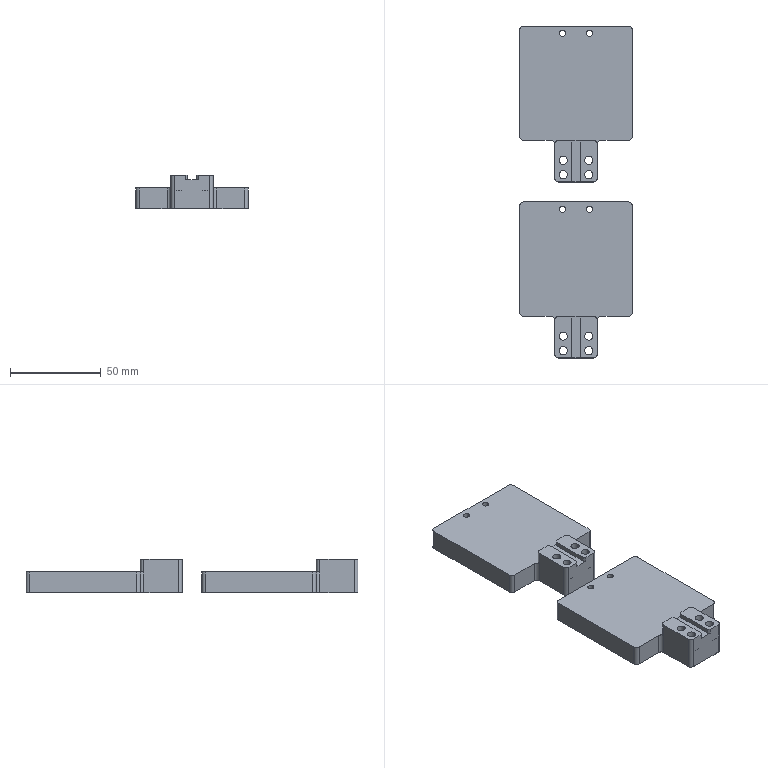NC program | NX | posted with a generic post | part box 62 x 183 x 18.5 mm
Lines 1 to 2420 of 4383, first 2274 of 2406 lines:
N10 G17 G21 G94 G90
(FLOOR_WALL , TOOL : D80)
N12 T19 M6
N14 G54
N16 G17 G0 G90 X229. Y31. S6500 M3
N18 G43 Z30. H19
N20 Z3.
N22 G94 G1 Z0. F1500.
N24 X226.
N26 X-43.
N28 X-46.
N30 Z3.
N32 G0 Z30.
N34 M5
(CAVITY_MILL , TOOL : D10)
N36 T15 M6
N38 G54
N40 G17 G0 G90 X84.33 Y-9.997 S9500 M3
N42 G43 Z30. H15
N44 Z1.026
N46 G94 G1 Z-0.974 F1000.
N48 X80.866 Y-3.997
N50 G3 X80. Y-3.497 R1.
N52 G1 X67.219 F3500.
N54 G2 X61. Y-6.3 R8.3
N56 G1 X2.
N58 G2 X-6.3 Y2. R8.3
N60 G1 Y60.
N62 G2 X2. Y68.3 R8.3
N64 G1 X61.
N66 G2 X67.219 Y65.497 R8.3
N68 G1 X90.7
N70 Y59.497
N72 Y45.599
N74 G3 X84. Y49. R8.3
N76 G1 X69.3
N78 Y59.497
N80 X90.7
N82 X86.2 Y54.997
N84 Y53.31
N86 G3 X84. Y53.5 R12.8
N88 G1 X73.8
N90 Y54.997
N92 X86.2
N94 X90.7 Y59.497
N96 Y65.497
N98 X92.781
N100 G2 X99. Y68.3 R8.3
N102 G1 X158.
N104 G2 X164.219 Y65.497 R8.3
N106 G1 X186.
N108 G2 X186.497 Y65. R0.497
N110 G1 Y49.
N112 X180.497
N114 X166.3
N116 Y59.497
N118 X180.497
N120 Y49.
N122 X175.997 Y53.5
N124 X170.8
N126 Y54.997
N128 X175.997
N130 Y53.5
N132 X180.497 Y49.
N134 X186.497
N136 Y46.919
N138 G2 X189.3 Y40.7 R8.3
N140 G1 Y21.3
N142 G2 X186.497 Y15.081 R8.3
N144 G1 Y-3.
N146 G2 X186. Y-3.497 R0.497
N148 G1 X166.3
N150 Y2.503
N152 Y13.
N154 X180.497
N156 Y2.503
N158 X166.3
N160 X170.8 Y7.003
N162 Y8.5
N164 X175.997
N166 Y7.003
N168 X170.8
N170 X166.3 Y2.503
N172 Y-3.497
N174 X164.219
N176 G2 X158. Y-6.3 R8.3
N178 G1 X99.
N180 G2 X92.781 Y-3.497 R8.3
N182 G1 X80.
N184 Y2.503
N186 X69.3
N188 Y13.
N190 X84.
N192 G3 X90.7 Y16.401 R8.3
N194 G1 X89.731 Y17.109
N196 G2 X84. Y14.2 R7.1
N198 G1 X68.1
N200 Y2.
N202 G2 X61. Y-5.1 R7.1
N204 G1 X2.
N206 G2 X-5.1 Y2. R7.1
N208 G1 Y60.
N210 G2 X2. Y67.1 R7.1
N212 G1 X61.
N214 G2 X68.1 Y60. R7.1
N216 G1 Y47.8
N218 X84.
N220 G2 X91.1 Y40.7 R7.1
N222 G1 Y21.3
N224 G2 X89.731 Y17.109 R7.1
N226 G1 X90.7 Y16.401
N228 Y2.503
N230 X91.9
N232 Y60.
N234 G2 X99. Y67.1 R7.1
N236 G1 X158.
N238 G2 X165.1 Y60. R7.1
N240 G1 Y47.8
N242 X181.
N244 G2 X188.1 Y40.7 R7.1
N246 G1 Y21.3
N248 G2 X181. Y14.2 R7.1
N250 G1 X165.1
N252 Y2.
N254 G2 X158. Y-5.1 R7.1
N256 G1 X99.
N258 G2 X91.9 Y2. R7.1
N260 G1 Y2.503
N262 X90.7
N264 X80.
N266 Y7.003
N268 X73.8
N270 Y8.5
N272 X84.
N274 G3 X86.2 Y8.69 R12.8
N276 G1 Y7.003
N278 X80.
N280 G3 X79.134 Y6.503 R1.
N282 G1 Z1.026
N284 G0 Z30.
N286 X84.33 Y-9.997
N288 Z0.053
N290 G1 Z-1.947 F1000.
N292 X80.866 Y-3.997
N294 G3 X80. Y-3.497 R1.
N296 G1 X67.219 F3500.
N298 G2 X61. Y-6.3 R8.3
N300 G1 X2.
N302 G2 X-6.3 Y2. R8.3
N304 G1 Y60.
N306 G2 X2. Y68.3 R8.3
N308 G1 X61.
N310 G2 X67.219 Y65.497 R8.3
N312 G1 X90.7
N314 Y59.497
N316 Y45.599
N318 G3 X84. Y49. R8.3
N320 G1 X69.3
N322 Y59.497
N324 X90.7
N326 X86.2 Y54.997
N328 Y53.31
N330 G3 X84. Y53.5 R12.8
N332 G1 X73.8
N334 Y54.997
N336 X86.2
N338 X90.7 Y59.497
N340 Y65.497
N342 X92.781
N344 G2 X99. Y68.3 R8.3
N346 G1 X158.
N348 G2 X164.219 Y65.497 R8.3
N350 G1 X186.
N352 G2 X186.497 Y65. R0.497
N354 G1 Y49.
N356 X180.497
N358 X166.3
N360 Y59.497
N362 X180.497
N364 Y49.
N366 X175.997 Y53.5
N368 X170.8
N370 Y54.997
N372 X175.997
N374 Y53.5
N376 X180.497 Y49.
N378 X186.497
N380 Y46.919
N382 G2 X189.3 Y40.7 R8.3
N384 G1 Y21.3
N386 G2 X186.497 Y15.081 R8.3
N388 G1 Y-3.
N390 G2 X186. Y-3.497 R0.497
N392 G1 X166.3
N394 Y2.503
N396 Y13.
N398 X180.497
N400 Y2.503
N402 X166.3
N404 X170.8 Y7.003
N406 Y8.5
N408 X175.997
N410 Y7.003
N412 X170.8
N414 X166.3 Y2.503
N416 Y-3.497
N418 X164.219
N420 G2 X158. Y-6.3 R8.3
N422 G1 X99.
N424 G2 X92.781 Y-3.497 R8.3
N426 G1 X80.
N428 Y2.503
N430 X69.3
N432 Y13.
N434 X84.
N436 G3 X90.7 Y16.401 R8.3
N438 G1 X89.731 Y17.109
N440 G2 X84. Y14.2 R7.1
N442 G1 X68.1
N444 Y2.
N446 G2 X61. Y-5.1 R7.1
N448 G1 X2.
N450 G2 X-5.1 Y2. R7.1
N452 G1 Y60.
N454 G2 X2. Y67.1 R7.1
N456 G1 X61.
N458 G2 X68.1 Y60. R7.1
N460 G1 Y47.8
N462 X84.
N464 G2 X91.1 Y40.7 R7.1
N466 G1 Y21.3
N468 G2 X89.731 Y17.109 R7.1
N470 G1 X90.7 Y16.401
N472 Y2.503
N474 X91.9
N476 Y60.
N478 G2 X99. Y67.1 R7.1
N480 G1 X158.
N482 G2 X165.1 Y60. R7.1
N484 G1 Y47.8
N486 X181.
N488 G2 X188.1 Y40.7 R7.1
N490 G1 Y21.3
N492 G2 X181. Y14.2 R7.1
N494 G1 X165.1
N496 Y2.
N498 G2 X158. Y-5.1 R7.1
N500 G1 X99.
N502 G2 X91.9 Y2. R7.1
N504 G1 Y2.503
N506 X90.7
N508 X80.
N510 Y7.003
N512 X73.8
N514 Y8.5
N516 X84.
N518 G3 X86.2 Y8.69 R12.8
N520 G1 Y7.003
N522 X80.
N524 G3 X79.134 Y6.503 R1.
N526 G1 Z0.053
N528 G0 X84.33 Y-9.997 Z-0.921
N530 G1 Z-2.921 F1000.
N532 X80.866 Y-3.997
N534 G3 X80. Y-3.497 R1.
N536 G1 X67.218 F3500.
N538 G2 X61. Y-6.3 R8.3
N540 G1 X2.
N542 G2 X-6.3 Y2. R8.3
N544 G1 Y60.
N546 G2 X2. Y68.3 R8.3
N548 G1 X61.
N550 G2 X67.218 Y65.497 R8.3
N552 G1 X90.7
N554 Y59.497
N556 Y45.599
N558 G3 X84. Y49. R8.3
N560 G1 X69.3
N562 Y59.497
N564 X90.7
N566 X86.2 Y54.997
N568 Y53.31
N570 G3 X84. Y53.5 R12.8
N572 G1 X73.8
N574 Y54.997
N576 X86.2
N578 X90.7 Y59.497
N580 Y65.497
N582 X92.782
N584 G2 X99. Y68.3 R8.3
N586 G1 X158.
N588 G2 X164.218 Y65.497 R8.3
N590 G1 X186.
N592 G2 X186.497 Y65. R0.497
N594 G1 Y49.
N596 X180.497
N598 X166.3
N600 Y59.497
N602 X180.497
N604 Y49.
N606 X175.997 Y53.5
N608 X170.8
N610 Y54.997
N612 X175.997
N614 Y53.5
N616 X180.497 Y49.
N618 X186.497
N620 Y46.918
N622 G2 X189.3 Y40.7 R8.3
N624 G1 Y21.3
N626 G2 X186.497 Y15.082 R8.3
N628 G1 Y-3.
N630 G2 X186. Y-3.497 R0.497
N632 G1 X166.3
N634 Y2.503
N636 Y13.
N638 X180.497
N640 Y2.503
N642 X166.3
N644 X170.8 Y7.003
N646 Y8.5
N648 X175.997
N650 Y7.003
N652 X170.8
N654 X166.3 Y2.503
N656 Y-3.497
N658 X164.218
N660 G2 X158. Y-6.3 R8.3
N662 G1 X99.
N664 G2 X92.782 Y-3.497 R8.3
N666 G1 X80.
N668 Y2.503
N670 X69.3
N672 Y13.
N674 X84.
N676 G3 X90.7 Y16.401 R8.3
N678 G1 X89.731 Y17.109
N680 G2 X84. Y14.2 R7.1
N682 G1 X68.1
N684 Y2.
N686 G2 X61. Y-5.1 R7.1
N688 G1 X2.
N690 G2 X-5.1 Y2. R7.1
N692 G1 Y60.
N694 G2 X2. Y67.1 R7.1
N696 G1 X61.
N698 G2 X68.1 Y60. R7.1
N700 G1 Y47.8
N702 X84.
N704 G2 X91.1 Y40.7 R7.1
N706 G1 Y21.3
N708 G2 X89.731 Y17.109 R7.1
N710 G1 X90.7 Y16.401
N712 Y2.503
N714 X91.9
N716 Y60.
N718 G2 X99. Y67.1 R7.1
N720 G1 X158.
N722 G2 X165.1 Y60. R7.1
N724 G1 Y47.8
N726 X181.
N728 G2 X188.1 Y40.7 R7.1
N730 G1 Y21.3
N732 G2 X181. Y14.2 R7.1
N734 G1 X165.1
N736 Y2.
N738 G2 X158. Y-5.1 R7.1
N740 G1 X99.
N742 G2 X91.9 Y2. R7.1
N744 G1 Y2.503
N746 X90.7
N748 X80.
N750 Y7.003
N752 X73.8
N754 Y8.5
N756 X84.
N758 G3 X86.2 Y8.69 R12.8
N760 G1 Y7.003
N762 X80.
N764 G3 X79.134 Y6.503 R1.
N766 G1 Z-0.921
N768 G0 X84.33 Y-9.998 Z-1.895
N770 G1 Z-3.895 F1000.
N772 X80.866 Y-3.998
N774 G3 X80. Y-3.498 R1.
N776 G1 X67.218 F3500.
N778 G2 X61. Y-6.3 R8.3
N780 G1 X2.
N782 G2 X-6.3 Y2. R8.3
N784 G1 Y60.
N786 G2 X2. Y68.3 R8.3
N788 G1 X61.
N790 G2 X67.218 Y65.498 R8.3
N792 G1 X90.7
N794 Y59.498
N796 Y45.599
N798 G3 X84. Y49. R8.3
N800 G1 X69.3
N802 Y59.498
N804 X90.7
N806 X86.2 Y54.998
N808 Y53.31
N810 G3 X84. Y53.5 R12.8
N812 G1 X73.8
N814 Y54.998
N816 X86.2
N818 X90.7 Y59.498
N820 Y65.498
N822 X92.782
N824 G2 X99. Y68.3 R8.3
N826 G1 X158.
N828 G2 X164.218 Y65.498 R8.3
N830 G1 X186.
N832 G2 X186.498 Y65. R0.497
N834 G1 Y49.
N836 X180.498
N838 X166.3
N840 Y59.498
N842 X180.498
N844 Y49.
N846 X175.998 Y53.5
N848 X170.8
N850 Y54.998
N852 X175.998
N854 Y53.5
N856 X180.498 Y49.
N858 X186.498
N860 Y46.918
N862 G2 X189.3 Y40.7 R8.3
N864 G1 Y21.3
N866 G2 X186.498 Y15.082 R8.3
N868 G1 Y-3.
N870 G2 X186. Y-3.498 R0.497
N872 G1 X166.3
N874 Y2.502
N876 Y13.
N878 X180.498
N880 Y2.502
N882 X166.3
N884 X170.8 Y7.002
N886 Y8.5
N888 X175.998
N890 Y7.002
N892 X170.8
N894 X166.3 Y2.502
N896 Y-3.498
N898 X164.218
N900 G2 X158. Y-6.3 R8.3
N902 G1 X99.
N904 G2 X92.782 Y-3.498 R8.3
N906 G1 X80.
N908 Y2.502
N910 X69.3
N912 Y13.
N914 X84.
N916 G3 X90.7 Y16.401 R8.3
N918 G1 X89.731 Y17.109
N920 G2 X84. Y14.2 R7.1
N922 G1 X68.1
N924 Y2.
N926 G2 X61. Y-5.1 R7.1
N928 G1 X2.
N930 G2 X-5.1 Y2. R7.1
N932 G1 Y60.
N934 G2 X2. Y67.1 R7.1
N936 G1 X61.
N938 G2 X68.1 Y60. R7.1
N940 G1 Y47.8
N942 X84.
N944 G2 X91.1 Y40.7 R7.1
N946 G1 Y21.3
N948 G2 X89.731 Y17.109 R7.1
N950 G1 X90.7 Y16.401
N952 Y2.502
N954 X91.9
N956 Y60.
N958 G2 X99. Y67.1 R7.1
N960 G1 X158.
N962 G2 X165.1 Y60. R7.1
N964 G1 Y47.8
N966 X181.
N968 G2 X188.1 Y40.7 R7.1
N970 G1 Y21.3
N972 G2 X181. Y14.2 R7.1
N974 G1 X165.1
N976 Y2.
N978 G2 X158. Y-5.1 R7.1
N980 G1 X99.
N982 G2 X91.9 Y2. R7.1
N984 G1 Y2.502
N986 X90.7
N988 X80.
N990 Y7.002
N992 X73.8
N994 Y8.5
N996 X84.
N998 G3 X86.2 Y8.69 R12.8
N1000 G1 Y7.002
N1002 X80.
N1004 G3 X79.134 Y6.502 R1.
N1006 G1 Z-1.895
N1008 G0 X84.33 Y-9.998 Z-2.868
N1010 G1 Z-4.868 F1000.
N1012 X80.866 Y-3.998
N1014 G3 X80. Y-3.498 R1.
N1016 G1 X67.218 F3500.
N1018 G2 X61. Y-6.3 R8.3
N1020 G1 X2.
N1022 G2 X-6.3 Y2. R8.3
N1024 G1 Y60.
N1026 G2 X2. Y68.3 R8.3
N1028 G1 X61.
N1030 G2 X67.218 Y65.498 R8.3
N1032 G1 X90.7
N1034 Y59.498
N1036 Y45.599
N1038 G3 X84. Y49. R8.3
N1040 G1 X69.3
N1042 Y59.498
N1044 X90.7
N1046 X86.2 Y54.998
N1048 Y53.31
N1050 G3 X84. Y53.5 R12.8
N1052 G1 X73.8
N1054 Y54.998
N1056 X86.2
N1058 X90.7 Y59.498
N1060 Y65.498
N1062 X92.782
N1064 G2 X99. Y68.3 R8.3
N1066 G1 X158.
N1068 G2 X164.218 Y65.498 R8.3
N1070 G1 X186.
N1072 G2 X186.498 Y65. R0.497
N1074 G1 Y49.
N1076 X180.498
N1078 X166.3
N1080 Y59.498
N1082 X180.498
N1084 Y49.
N1086 X175.998 Y53.5
N1088 X170.8
N1090 Y54.998
N1092 X175.998
N1094 Y53.5
N1096 X180.498 Y49.
N1098 X186.498
N1100 Y46.918
N1102 G2 X189.3 Y40.7 R8.3
N1104 G1 Y21.3
N1106 G2 X186.498 Y15.082 R8.3
N1108 G1 Y-3.
N1110 G2 X186. Y-3.498 R0.497
N1112 G1 X166.3
N1114 Y2.502
N1116 Y13.
N1118 X180.498
N1120 Y2.502
N1122 X166.3
N1124 X170.8 Y7.002
N1126 Y8.5
N1128 X175.998
N1130 Y7.002
N1132 X170.8
N1134 X166.3 Y2.502
N1136 Y-3.498
N1138 X164.218
N1140 G2 X158. Y-6.3 R8.3
N1142 G1 X99.
N1144 G2 X92.782 Y-3.498 R8.3
N1146 G1 X80.
N1148 Y2.502
N1150 X69.3
N1152 Y13.
N1154 X84.
N1156 G3 X90.7 Y16.401 R8.3
N1158 G1 X89.731 Y17.109
N1160 G2 X84. Y14.2 R7.1
N1162 G1 X68.1
N1164 Y2.
N1166 G2 X61. Y-5.1 R7.1
N1168 G1 X2.
N1170 G2 X-5.1 Y2. R7.1
N1172 G1 Y60.
N1174 G2 X2. Y67.1 R7.1
N1176 G1 X61.
N1178 G2 X68.1 Y60. R7.1
N1180 G1 Y47.8
N1182 X84.
N1184 G2 X91.1 Y40.7 R7.1
N1186 G1 Y21.3
N1188 G2 X89.731 Y17.109 R7.1
N1190 G1 X90.7 Y16.401
N1192 Y2.502
N1194 X91.9
N1196 Y60.
N1198 G2 X99. Y67.1 R7.1
N1200 G1 X158.
N1202 G2 X165.1 Y60. R7.1
N1204 G1 Y47.8
N1206 X181.
N1208 G2 X188.1 Y40.7 R7.1
N1210 G1 Y21.3
N1212 G2 X181. Y14.2 R7.1
N1214 G1 X165.1
N1216 Y2.
N1218 G2 X158. Y-5.1 R7.1
N1220 G1 X99.
N1222 G2 X91.9 Y2. R7.1
N1224 G1 Y2.502
N1226 X90.7
N1228 X80.
N1230 Y7.002
N1232 X73.8
N1234 Y8.5
N1236 X84.
N1238 G3 X86.2 Y8.69 R12.8
N1240 G1 Y7.002
N1242 X80.
N1244 G3 X79.134 Y6.502 R1.
N1246 G1 Z-2.868
N1248 G0 X84.33 Y-9.998 Z-3.842
N1250 G1 Z-5.842 F1000.
N1252 X80.866 Y-3.998
N1254 G3 X80. Y-3.498 R1.
N1256 G1 X67.218 F3500.
N1258 G2 X61. Y-6.3 R8.3
N1260 G1 X2.
N1262 G2 X-6.3 Y2. R8.3
N1264 G1 Y60.
N1266 G2 X2. Y68.3 R8.3
N1268 G1 X61.
N1270 G2 X67.218 Y65.498 R8.3
N1272 G1 X90.7
N1274 Y59.498
N1276 Y45.599
N1278 G3 X84. Y49. R8.3
N1280 G1 X69.3
N1282 Y59.498
N1284 X90.7
N1286 X86.2 Y54.998
N1288 Y53.31
N1290 G3 X84. Y53.5 R12.8
N1292 G1 X73.8
N1294 Y54.998
N1296 X86.2
N1298 X90.7 Y59.498
N1300 Y65.498
N1302 X92.782
N1304 G2 X99. Y68.3 R8.3
N1306 G1 X158.
N1308 G2 X164.218 Y65.498 R8.3
N1310 G1 X186.
N1312 G2 X186.498 Y65. R0.498
N1314 G1 Y49.
N1316 X180.498
N1318 X166.3
N1320 Y59.498
N1322 X180.498
N1324 Y49.
N1326 X175.998 Y53.5
N1328 X170.8
N1330 Y54.998
N1332 X175.998
N1334 Y53.5
N1336 X180.498 Y49.
N1338 X186.498
N1340 Y46.918
N1342 G2 X189.3 Y40.7 R8.3
N1344 G1 Y21.3
N1346 G2 X186.498 Y15.082 R8.3
N1348 G1 Y-3.
N1350 G2 X186. Y-3.498 R0.498
N1352 G1 X166.3
N1354 Y2.502
N1356 Y13.
N1358 X180.498
N1360 Y2.502
N1362 X166.3
N1364 X170.8 Y7.002
N1366 Y8.5
N1368 X175.998
N1370 Y7.002
N1372 X170.8
N1374 X166.3 Y2.502
N1376 Y-3.498
N1378 X164.218
N1380 G2 X158. Y-6.3 R8.3
N1382 G1 X99.
N1384 G2 X92.782 Y-3.498 R8.3
N1386 G1 X80.
N1388 Y2.502
N1390 X69.3
N1392 Y13.
N1394 X84.
N1396 G3 X90.7 Y16.401 R8.3
N1398 G1 X89.731 Y17.109
N1400 G2 X84. Y14.2 R7.1
N1402 G1 X68.1
N1404 Y2.
N1406 G2 X61. Y-5.1 R7.1
N1408 G1 X2.
N1410 G2 X-5.1 Y2. R7.1
N1412 G1 Y60.
N1414 G2 X2. Y67.1 R7.1
N1416 G1 X61.
N1418 G2 X68.1 Y60. R7.1
N1420 G1 Y47.8
N1422 X84.
N1424 G2 X91.1 Y40.7 R7.1
N1426 G1 Y21.3
N1428 G2 X89.731 Y17.109 R7.1
N1430 G1 X90.7 Y16.401
N1432 Y2.502
N1434 X91.9
N1436 Y60.
N1438 G2 X99. Y67.1 R7.1
N1440 G1 X158.
N1442 G2 X165.1 Y60. R7.1
N1444 G1 Y47.8
N1446 X181.
N1448 G2 X188.1 Y40.7 R7.1
N1450 G1 Y21.3
N1452 G2 X181. Y14.2 R7.1
N1454 G1 X165.1
N1456 Y2.
N1458 G2 X158. Y-5.1 R7.1
N1460 G1 X99.
N1462 G2 X91.9 Y2. R7.1
N1464 G1 Y2.502
N1466 X90.7
N1468 X80.
N1470 Y7.002
N1472 X73.8
N1474 Y8.5
N1476 X84.
N1478 G3 X86.2 Y8.69 R12.8
N1480 G1 Y7.002
N1482 X80.
N1484 G3 X79.134 Y6.502 R1.
N1486 G1 Z-3.842
N1488 G0 X84.33 Y-9.998 Z-4.816
N1490 G1 Z-6.816 F1000.
N1492 X80.866 Y-3.998
N1494 G3 X80. Y-3.498 R1.
N1496 G1 X67.218 F3500.
N1498 G2 X61. Y-6.3 R8.3
N1500 G1 X2.
N1502 G2 X-6.3 Y2. R8.3
N1504 G1 Y60.
N1506 G2 X2. Y68.3 R8.3
N1508 G1 X61.
N1510 G2 X67.218 Y65.498 R8.3
N1512 G1 X90.7
N1514 Y59.498
N1516 Y45.599
N1518 G3 X84. Y49. R8.3
N1520 G1 X69.3
N1522 Y59.498
N1524 X90.7
N1526 X86.2 Y54.998
N1528 Y53.31
N1530 G3 X84. Y53.5 R12.8
N1532 G1 X73.8
N1534 Y54.998
N1536 X86.2
N1538 X90.7 Y59.498
N1540 Y65.498
N1542 X92.782
N1544 G2 X99. Y68.3 R8.3
N1546 G1 X158.
N1548 G2 X164.218 Y65.498 R8.3
N1550 G1 X186.
N1552 G2 X186.498 Y65. R0.498
N1554 G1 Y49.
N1556 X180.498
N1558 X166.3
N1560 Y59.498
N1562 X180.498
N1564 Y49.
N1566 X175.998 Y53.5
N1568 X170.8
N1570 Y54.998
N1572 X175.998
N1574 Y53.5
N1576 X180.498 Y49.
N1578 X186.498
N1580 Y46.918
N1582 G2 X189.3 Y40.7 R8.3
N1584 G1 Y21.3
N1586 G2 X186.498 Y15.082 R8.3
N1588 G1 Y-3.
N1590 G2 X186. Y-3.498 R0.498
N1592 G1 X166.3
N1594 Y2.502
N1596 Y13.
N1598 X180.498
N1600 Y2.502
N1602 X166.3
N1604 X170.8 Y7.002
N1606 Y8.5
N1608 X175.998
N1610 Y7.002
N1612 X170.8
N1614 X166.3 Y2.502
N1616 Y-3.498
N1618 X164.218
N1620 G2 X158. Y-6.3 R8.3
N1622 G1 X99.
N1624 G2 X92.782 Y-3.498 R8.3
N1626 G1 X80.
N1628 Y2.502
N1630 X69.3
N1632 Y13.
N1634 X84.
N1636 G3 X90.7 Y16.401 R8.3
N1638 G1 X89.731 Y17.109
N1640 G2 X84. Y14.2 R7.1
N1642 G1 X68.1
N1644 Y2.
N1646 G2 X61. Y-5.1 R7.1
N1648 G1 X2.
N1650 G2 X-5.1 Y2. R7.1
N1652 G1 Y60.
N1654 G2 X2. Y67.1 R7.1
N1656 G1 X61.
N1658 G2 X68.1 Y60. R7.1
N1660 G1 Y47.8
N1662 X84.
N1664 G2 X91.1 Y40.7 R7.1
N1666 G1 Y21.3
N1668 G2 X89.731 Y17.109 R7.1
N1670 G1 X90.7 Y16.401
N1672 Y2.502
N1674 X91.9
N1676 Y60.
N1678 G2 X99. Y67.1 R7.1
N1680 G1 X158.
N1682 G2 X165.1 Y60. R7.1
N1684 G1 Y47.8
N1686 X181.
N1688 G2 X188.1 Y40.7 R7.1
N1690 G1 Y21.3
N1692 G2 X181. Y14.2 R7.1
N1694 G1 X165.1
N1696 Y2.
N1698 G2 X158. Y-5.1 R7.1
N1700 G1 X99.
N1702 G2 X91.9 Y2. R7.1
N1704 G1 Y2.502
N1706 X90.7
N1708 X80.
N1710 Y7.002
N1712 X73.8
N1714 Y8.5
N1716 X84.
N1718 G3 X86.2 Y8.69 R12.8
N1720 G1 Y7.002
N1722 X80.
N1724 G3 X79.134 Y6.502 R1.
N1726 G1 Z-4.816
N1728 G0 X84.33 Y-9.998 Z-5.789
N1730 G1 Z-7.789 F1000.
N1732 X80.866 Y-3.998
N1734 G3 X80. Y-3.498 R1.
N1736 G1 X67.218 F3500.
N1738 G2 X61. Y-6.3 R8.3
N1740 G1 X2.
N1742 G2 X-6.3 Y2. R8.3
N1744 G1 Y60.
N1746 G2 X2. Y68.3 R8.3
N1748 G1 X61.
N1750 G2 X67.218 Y65.498 R8.3
N1752 G1 X90.7
N1754 Y59.498
N1756 Y45.599
N1758 G3 X84. Y49. R8.3
N1760 G1 X69.3
N1762 Y59.498
N1764 X90.7
N1766 X86.2 Y54.998
N1768 Y53.31
N1770 G3 X84. Y53.5 R12.8
N1772 G1 X73.8
N1774 Y54.998
N1776 X86.2
N1778 X90.7 Y59.498
N1780 Y65.498
N1782 X92.782
N1784 G2 X99. Y68.3 R8.3
N1786 G1 X158.
N1788 G2 X164.218 Y65.498 R8.3
N1790 G1 X186.
N1792 G2 X186.498 Y65. R0.498
N1794 G1 Y49.
N1796 X180.498
N1798 X166.3
N1800 Y59.498
N1802 X180.498
N1804 Y49.
N1806 X175.998 Y53.5
N1808 X170.8
N1810 Y54.998
N1812 X175.998
N1814 Y53.5
N1816 X180.498 Y49.
N1818 X186.498
N1820 Y46.918
N1822 G2 X189.3 Y40.7 R8.3
N1824 G1 Y21.3
N1826 G2 X186.498 Y15.082 R8.3
N1828 G1 Y-3.
N1830 G2 X186. Y-3.498 R0.498
N1832 G1 X166.3
N1834 Y2.502
N1836 Y13.
N1838 X180.498
N1840 Y2.502
N1842 X166.3
N1844 X170.8 Y7.002
N1846 Y8.5
N1848 X175.998
N1850 Y7.002
N1852 X170.8
N1854 X166.3 Y2.502
N1856 Y-3.498
N1858 X164.218
N1860 G2 X158. Y-6.3 R8.3
N1862 G1 X99.
N1864 G2 X92.782 Y-3.498 R8.3
N1866 G1 X80.
N1868 Y2.502
N1870 X69.3
N1872 Y13.
N1874 X84.
N1876 G3 X90.7 Y16.401 R8.3
N1878 G1 X89.731 Y17.109
N1880 G2 X84. Y14.2 R7.1
N1882 G1 X68.1
N1884 Y2.
N1886 G2 X61. Y-5.1 R7.1
N1888 G1 X2.
N1890 G2 X-5.1 Y2. R7.1
N1892 G1 Y60.
N1894 G2 X2. Y67.1 R7.1
N1896 G1 X61.
N1898 G2 X68.1 Y60. R7.1
N1900 G1 Y47.8
N1902 X84.
N1904 G2 X91.1 Y40.7 R7.1
N1906 G1 Y21.3
N1908 G2 X89.731 Y17.109 R7.1
N1910 G1 X90.7 Y16.401
N1912 Y2.502
N1914 X91.9
N1916 Y60.
N1918 G2 X99. Y67.1 R7.1
N1920 G1 X158.
N1922 G2 X165.1 Y60. R7.1
N1924 G1 Y47.8
N1926 X181.
N1928 G2 X188.1 Y40.7 R7.1
N1930 G1 Y21.3
N1932 G2 X181. Y14.2 R7.1
N1934 G1 X165.1
N1936 Y2.
N1938 G2 X158. Y-5.1 R7.1
N1940 G1 X99.
N1942 G2 X91.9 Y2. R7.1
N1944 G1 Y2.502
N1946 X90.7
N1948 X80.
N1950 Y7.002
N1952 X73.8
N1954 Y8.5
N1956 X84.
N1958 G3 X86.2 Y8.69 R12.8
N1960 G1 Y7.002
N1962 X80.
N1964 G3 X79.134 Y6.502 R1.
N1966 G1 Z-5.789
N1968 G0 X84.33 Y-9.998 Z-6.763
N1970 G1 Z-8.763 F1000.
N1972 X80.866 Y-3.998
N1974 G3 X80. Y-3.498 R1.
N1976 G1 X67.218 F3500.
N1978 G2 X61. Y-6.3 R8.3
N1980 G1 X2.
N1982 G2 X-6.3 Y2. R8.3
N1984 G1 Y60.
N1986 G2 X2. Y68.3 R8.3
N1988 G1 X61.
N1990 G2 X67.218 Y65.498 R8.3
N1992 G1 X90.7
N1994 Y59.498
N1996 Y45.599
N1998 G3 X84. Y49. R8.3
N2000 G1 X69.3
N2002 Y59.498
N2004 X90.7
N2006 X86.2 Y54.998
N2008 Y53.31
N2010 G3 X84. Y53.5 R12.8
N2012 G1 X73.8
N2014 Y54.998
N2016 X86.2
N2018 X90.7 Y59.498
N2020 Y65.498
N2022 X92.782
N2024 G2 X99. Y68.3 R8.3
N2026 G1 X158.
N2028 G2 X164.218 Y65.498 R8.3
N2030 G1 X186.
N2032 G2 X186.498 Y65. R0.498
N2034 G1 Y49.
N2036 X180.498
N2038 X166.3
N2040 Y59.498
N2042 X180.498
N2044 Y49.
N2046 X175.998 Y53.5
N2048 X170.8
N2050 Y54.998
N2052 X175.998
N2054 Y53.5
N2056 X180.498 Y49.
N2058 X186.498
N2060 Y46.918
N2062 G2 X189.3 Y40.7 R8.3
N2064 G1 Y21.3
N2066 G2 X186.498 Y15.082 R8.3
N2068 G1 Y-3.
N2070 G2 X186. Y-3.498 R0.498
N2072 G1 X166.3
N2074 Y2.502
N2076 Y13.
N2078 X180.498
N2080 Y2.502
N2082 X166.3
N2084 X170.8 Y7.002
N2086 Y8.5
N2088 X175.998
N2090 Y7.002
N2092 X170.8
N2094 X166.3 Y2.502
N2096 Y-3.498
N2098 X164.218
N2100 G2 X158. Y-6.3 R8.3
N2102 G1 X99.
N2104 G2 X92.782 Y-3.498 R8.3
N2106 G1 X80.
N2108 Y2.502
N2110 X69.3
N2112 Y13.
N2114 X84.
N2116 G3 X90.7 Y16.401 R8.3
N2118 G1 X89.731 Y17.109
N2120 G2 X84. Y14.2 R7.1
N2122 G1 X68.1
N2124 Y2.
N2126 G2 X61. Y-5.1 R7.1
N2128 G1 X2.
N2130 G2 X-5.1 Y2. R7.1
N2132 G1 Y60.
N2134 G2 X2. Y67.1 R7.1
N2136 G1 X61.
N2138 G2 X68.1 Y60. R7.1
N2140 G1 Y47.8
N2142 X84.
N2144 G2 X91.1 Y40.7 R7.1
N2146 G1 Y21.3
N2148 G2 X89.731 Y17.109 R7.1
N2150 G1 X90.7 Y16.401
N2152 Y2.502
N2154 X91.9
N2156 Y60.
N2158 G2 X99. Y67.1 R7.1
N2160 G1 X158.
N2162 G2 X165.1 Y60. R7.1
N2164 G1 Y47.8
N2166 X181.
N2168 G2 X188.1 Y40.7 R7.1
N2170 G1 Y21.3
N2172 G2 X181. Y14.2 R7.1
N2174 G1 X165.1
N2176 Y2.
N2178 G2 X158. Y-5.1 R7.1
N2180 G1 X99.
N2182 G2 X91.9 Y2. R7.1
N2184 G1 Y2.502
N2186 X90.7
N2188 X80.
N2190 Y7.002
N2192 X73.8
N2194 Y8.5
N2196 X84.
N2198 G3 X86.2 Y8.69 R12.8
N2200 G1 Y7.002
N2202 X80.
N2204 G3 X79.134 Y6.502 R1.
N2206 G1 Z-6.763
N2208 G0 X84.33 Y-9.999 Z-7.737
N2210 G1 Z-9.737 F1000.
N2212 X80.866 Y-3.999
N2214 G3 X80. Y-3.499 R1.
N2216 G1 X67.217 F3500.
N2218 G2 X61. Y-6.3 R8.3
N2220 G1 X2.
N2222 G2 X-6.3 Y2. R8.3
N2224 G1 Y60.
N2226 G2 X2. Y68.3 R8.3
N2228 G1 X61.
N2230 G2 X67.217 Y65.499 R8.3
N2232 G1 X90.7
N2234 Y59.499
N2236 Y45.599
N2238 G3 X84. Y49. R8.3
N2240 G1 X69.3
N2242 Y59.499
N2244 X90.7
N2246 X86.2 Y54.999
N2248 Y53.31
N2250 G3 X84. Y53.5 R12.8
N2252 G1 X73.8
N2254 Y54.999
N2256 X86.2
N2258 X90.7 Y59.499
N2260 Y65.499
N2262 X92.783
N2264 G2 X99. Y68.3 R8.3
N2266 G1 X158.
N2268 G2 X164.217 Y65.499 R8.3
N2270 G1 X186.
N2272 G2 X186.499 Y65. R0.498
N2274 G1 Y49.
N2276 X180.499
N2278 X166.3
N2280 Y59.499
N2282 X180.499
N2284 Y49.
N2286 X175.999 Y53.5
N2288 X170.8
N2290 Y54.999
N2292 X175.999
N2294 Y53.5
N2296 X180.499 Y49.
N2298 X186.499
N2300 Y46.917
N2302 G2 X189.3 Y40.7 R8.3
N2304 G1 Y21.3
N2306 G2 X186.499 Y15.083 R8.3
N2308 G1 Y-3.
N2310 G2 X186. Y-3.499 R0.498
N2312 G1 X166.3
N2314 Y2.501
N2316 Y13.
N2318 X180.499
N2320 Y2.501
N2322 X166.3
N2324 X170.8 Y7.001
N2326 Y8.5
N2328 X175.999
N2330 Y7.001
N2332 X170.8
N2334 X166.3 Y2.501
N2336 Y-3.499
N2338 X164.217
N2340 G2 X158. Y-6.3 R8.3
N2342 G1 X99.
N2344 G2 X92.783 Y-3.499 R8.3
N2346 G1 X80.
N2348 Y2.501
N2350 X69.3
N2352 Y13.
N2354 X84.
N2356 G3 X90.7 Y16.401 R8.3
N2358 G1 X89.731 Y17.109
N2360 G2 X84. Y14.2 R7.1
N2362 G1 X68.1
N2364 Y2.
N2366 G2 X61. Y-5.1 R7.1
N2368 G1 X2.
N2370 G2 X-5.1 Y2. R7.1
N2372 G1 Y60.
N2374 G2 X2. Y67.1 R7.1
N2376 G1 X61.
N2378 G2 X68.1 Y60. R7.1
N2380 G1 Y47.8
N2382 X84.
N2384 G2 X91.1 Y40.7 R7.1
N2386 G1 Y21.3
N2388 G2 X89.731 Y17.109 R7.1
N2390 G1 X90.7 Y16.401
N2392 Y2.501
N2394 X91.9
N2396 Y60.
N2398 G2 X99. Y67.1 R7.1
N2400 G1 X158.
N2402 G2 X165.1 Y60. R7.1
N2404 G1 Y47.8
N2406 X181.
N2408 G2 X188.1 Y40.7 R7.1
N2410 G1 Y21.3
N2412 G2 X181. Y14.2 R7.1
N2414 G1 X165.1
N2416 Y2.
N2418 G2 X158. Y-5.1 R7.1
N2420 G1 X99.
N2422 G2 X91.9 Y2. R7.1
N2424 G1 Y2.501
N2426 X90.7
N2428 X80.
N2430 Y7.001
N2432 X73.8
N2434 Y8.5
N2436 X84.
N2438 G3 X86.2 Y8.69 R12.8
N2440 G1 Y7.001
N2442 X80.
N2444 G3 X79.134 Y6.501 R1.
N2446 G1 Z-7.737
N2448 G0 X84.33 Y-9.999 Z-8.711
N2450 G1 Z-10.711 F1000.
N2452 X80.866 Y-3.999
N2454 G3 X80. Y-3.499 R1.
N2456 G1 X67.217 F3500.
N2458 G2 X61. Y-6.3 R8.3
N2460 G1 X2.
N2462 G2 X-6.3 Y2. R8.3
N2464 G1 Y60.
N2466 G2 X2. Y68.3 R8.3
N2468 G1 X61.
N2470 G2 X67.217 Y65.499 R8.3
N2472 G1 X90.7
N2474 Y59.499
N2476 Y45.599
N2478 G3 X84. Y49. R8.3
N2480 G1 X69.3
N2482 Y59.499
N2484 X90.7
N2486 X86.2 Y54.999
N2488 Y53.31
N2490 G3 X84. Y53.5 R12.8
N2492 G1 X73.8
N2494 Y54.999
N2496 X86.2
N2498 X90.7 Y59.499
N2500 Y65.499
N2502 X92.783
N2504 G2 X99. Y68.3 R8.3
N2506 G1 X158.
N2508 G2 X164.217 Y65.499 R8.3
N2510 G1 X186.
N2512 G2 X186.499 Y65. R0.498
N2514 G1 Y49.
N2516 X180.499
N2518 X166.3
N2520 Y59.499
N2522 X180.499
N2524 Y49.
N2526 X175.999 Y53.5
N2528 X170.8
N2530 Y54.999
N2532 X175.999
N2534 Y53.5
N2536 X180.499 Y49.
N2538 X186.499
N2540 Y46.917
N2542 G2 X189.3 Y40.7 R8.3
N2544 G1 Y21.3
N2546 G2 X186.499 Y15.083 R8.3
N2548 G1 Y-3.
N2550 G2 X186. Y-3.499 R0.498
N2552 G1 X166.3
N2554 Y2.501
N2556 Y13.
N2558 X180.499
N2560 Y2.501
N2562 X166.3
N2564 X170.8 Y7.001
N2566 Y8.5
N2568 X175.999
N2570 Y7.001
N2572 X170.8
N2574 X166.3 Y2.501
N2576 Y-3.499
N2578 X164.217
N2580 G2 X158. Y-6.3 R8.3
N2582 G1 X99.
N2584 G2 X92.783 Y-3.499 R8.3
N2586 G1 X80.
N2588 Y2.501
N2590 X69.3
N2592 Y13.
N2594 X84.
N2596 G3 X90.7 Y16.401 R8.3
N2598 G1 X89.731 Y17.109
N2600 G2 X84. Y14.2 R7.1
N2602 G1 X68.1
N2604 Y2.
N2606 G2 X61. Y-5.1 R7.1
N2608 G1 X2.
N2610 G2 X-5.1 Y2. R7.1
N2612 G1 Y60.
N2614 G2 X2. Y67.1 R7.1
N2616 G1 X61.
N2618 G2 X68.1 Y60. R7.1
N2620 G1 Y47.8
N2622 X84.
N2624 G2 X91.1 Y40.7 R7.1
N2626 G1 Y21.3
N2628 G2 X89.731 Y17.109 R7.1
N2630 G1 X90.7 Y16.401
N2632 Y2.501
N2634 X91.9
N2636 Y60.
N2638 G2 X99. Y67.1 R7.1
N2640 G1 X158.
N2642 G2 X165.1 Y60. R7.1
N2644 G1 Y47.8
N2646 X181.
N2648 G2 X188.1 Y40.7 R7.1
N2650 G1 Y21.3
N2652 G2 X181. Y14.2 R7.1
N2654 G1 X165.1
N2656 Y2.
N2658 G2 X158. Y-5.1 R7.1
N2660 G1 X99.
N2662 G2 X91.9 Y2. R7.1
N2664 G1 Y2.501
N2666 X90.7
N2668 X80.
N2670 Y7.001
N2672 X73.8
N2674 Y8.5
N2676 X84.
N2678 G3 X86.2 Y8.69 R12.8
N2680 G1 Y7.001
N2682 X80.
N2684 G3 X79.134 Y6.501 R1.
N2686 G1 Z-8.711
N2688 G0 X84.33 Y-9.999 Z-9.684
N2690 G1 Z-11.684 F1000.
N2692 X80.866 Y-3.999
N2694 G3 X80. Y-3.499 R1.
N2696 G1 X67.217 F3500.
N2698 G2 X61. Y-6.3 R8.3
N2700 G1 X2.
N2702 G2 X-6.3 Y2. R8.3
N2704 G1 Y60.
N2706 G2 X2. Y68.3 R8.3
N2708 G1 X61.
N2710 G2 X67.217 Y65.499 R8.3
N2712 G1 X90.7
N2714 Y59.499
N2716 Y45.599
N2718 G3 X84. Y49. R8.3
N2720 G1 X69.3
N2722 Y59.499
N2724 X90.7
N2726 X86.2 Y54.999
N2728 Y53.31
N2730 G3 X84. Y53.5 R12.8
N2732 G1 X73.8
N2734 Y54.999
N2736 X86.2
N2738 X90.7 Y59.499
N2740 Y65.499
N2742 X92.783
N2744 G2 X99. Y68.3 R8.3
N2746 G1 X158.
N2748 G2 X164.217 Y65.499 R8.3
N2750 G1 X186.
N2752 G2 X186.499 Y65. R0.499
N2754 G1 Y49.
N2756 X180.499
N2758 X166.3
N2760 Y59.499
N2762 X180.499
N2764 Y49.
N2766 X175.999 Y53.5
N2768 X170.8
N2770 Y54.999
N2772 X175.999
N2774 Y53.5
N2776 X180.499 Y49.
N2778 X186.499
N2780 Y46.917
N2782 G2 X189.3 Y40.7 R8.3
N2784 G1 Y21.3
N2786 G2 X186.499 Y15.083 R8.3
N2788 G1 Y-3.
N2790 G2 X186. Y-3.499 R0.499
N2792 G1 X166.3
N2794 Y2.501
N2796 Y13.
N2798 X180.499
N2800 Y2.501
N2802 X166.3
N2804 X170.8 Y7.001
N2806 Y8.5
N2808 X175.999
N2810 Y7.001
N2812 X170.8
N2814 X166.3 Y2.501
N2816 Y-3.499
N2818 X164.217
N2820 G2 X158. Y-6.3 R8.3
N2822 G1 X99.
N2824 G2 X92.783 Y-3.499 R8.3
N2826 G1 X80.
N2828 Y2.501
N2830 X69.3
N2832 Y13.
N2834 X84.
N2836 G3 X90.7 Y16.401 R8.3
N2838 G1 X89.731 Y17.109
N2840 G2 X84. Y14.2 R7.1
N2842 G1 X68.1
N2844 Y2.
N2846 G2 X61. Y-5.1 R7.1
N2848 G1 X2.
N2850 G2 X-5.1 Y2. R7.1
N2852 G1 Y60.
N2854 G2 X2. Y67.1 R7.1
N2856 G1 X61.
N2858 G2 X68.1 Y60. R7.1
N2860 G1 Y47.8
N2862 X84.
N2864 G2 X91.1 Y40.7 R7.1
N2866 G1 Y21.3
N2868 G2 X89.731 Y17.109 R7.1
N2870 G1 X90.7 Y16.401
N2872 Y2.501
N2874 X91.9
N2876 Y60.
N2878 G2 X99. Y67.1 R7.1
N2880 G1 X158.
N2882 G2 X165.1 Y60. R7.1
N2884 G1 Y47.8
N2886 X181.
N2888 G2 X188.1 Y40.7 R7.1
N2890 G1 Y21.3
N2892 G2 X181. Y14.2 R7.1
N2894 G1 X165.1
N2896 Y2.
N2898 G2 X158. Y-5.1 R7.1
N2900 G1 X99.
N2902 G2 X91.9 Y2. R7.1
N2904 G1 Y2.501
N2906 X90.7
N2908 X80.
N2910 Y7.001
N2912 X73.8
N2914 Y8.5
N2916 X84.
N2918 G3 X86.2 Y8.69 R12.8
N2920 G1 Y7.001
N2922 X80.
N2924 G3 X79.134 Y6.501 R1.
N2926 G1 Z-9.684
N2928 G0 X84.33 Y-9.999 Z-10.658
N2930 G1 Z-12.658 F1000.
N2932 X80.866 Y-3.999
N2934 G3 X80. Y-3.499 R1.
N2936 G1 X67.217 F3500.
N2938 G2 X61. Y-6.3 R8.3
N2940 G1 X2.
N2942 G2 X-6.3 Y2. R8.3
N2944 G1 Y60.
N2946 G2 X2. Y68.3 R8.3
N2948 G1 X61.
N2950 G2 X67.217 Y65.499 R8.3
N2952 G1 X90.7
N2954 Y59.499
N2956 Y45.599
N2958 G3 X84. Y49. R8.3
N2960 G1 X69.3
N2962 Y59.499
N2964 X90.7
N2966 X86.2 Y54.999
N2968 Y53.31
N2970 G3 X84. Y53.5 R12.8
N2972 G1 X73.8
N2974 Y54.999
N2976 X86.2
N2978 X90.7 Y59.499
N2980 Y65.499
N2982 X92.783
N2984 G2 X99. Y68.3 R8.3
N2986 G1 X158.
N2988 G2 X164.217 Y65.499 R8.3
N2990 G1 X186.
N2992 G2 X186.499 Y65. R0.499
N2994 G1 Y49.
N2996 X180.499
N2998 X166.3
N3000 Y59.499
N3002 X180.499
N3004 Y49.
N3006 X175.999 Y53.5
N3008 X170.8
N3010 Y54.999
N3012 X175.999
N3014 Y53.5
N3016 X180.499 Y49.
N3018 X186.499
N3020 Y46.917
N3022 G2 X189.3 Y40.7 R8.3
N3024 G1 Y21.3
N3026 G2 X186.499 Y15.083 R8.3
N3028 G1 Y-3.
N3030 G2 X186. Y-3.499 R0.499
N3032 G1 X166.3
N3034 Y2.501
N3036 Y13.
N3038 X180.499
N3040 Y2.501
N3042 X166.3
N3044 X170.8 Y7.001
N3046 Y8.5
N3048 X175.999
N3050 Y7.001
N3052 X170.8
N3054 X166.3 Y2.501
N3056 Y-3.499
N3058 X164.217
N3060 G2 X158. Y-6.3 R8.3
N3062 G1 X99.
N3064 G2 X92.783 Y-3.499 R8.3
N3066 G1 X80.
N3068 Y2.501
N3070 X69.3
N3072 Y13.
N3074 X84.
N3076 G3 X90.7 Y16.401 R8.3
N3078 G1 X89.731 Y17.109
N3080 G2 X84. Y14.2 R7.1
N3082 G1 X68.1
N3084 Y2.
N3086 G2 X61. Y-5.1 R7.1
N3088 G1 X2.
N3090 G2 X-5.1 Y2. R7.1
N3092 G1 Y60.
N3094 G2 X2. Y67.1 R7.1
N3096 G1 X61.
N3098 G2 X68.1 Y60. R7.1
N3100 G1 Y47.8
N3102 X84.
N3104 G2 X91.1 Y40.7 R7.1
N3106 G1 Y21.3
N3108 G2 X89.731 Y17.109 R7.1
N3110 G1 X90.7 Y16.401
N3112 Y2.501
N3114 X91.9
N3116 Y60.
N3118 G2 X99. Y67.1 R7.1
N3120 G1 X158.
N3122 G2 X165.1 Y60. R7.1
N3124 G1 Y47.8
N3126 X181.
N3128 G2 X188.1 Y40.7 R7.1
N3130 G1 Y21.3
N3132 G2 X181. Y14.2 R7.1
N3134 G1 X165.1
N3136 Y2.
N3138 G2 X158. Y-5.1 R7.1
N3140 G1 X99.
N3142 G2 X91.9 Y2. R7.1
N3144 G1 Y2.501
N3146 X90.7
N3148 X80.
N3150 Y7.001
N3152 X73.8
N3154 Y8.5
N3156 X84.
N3158 G3 X86.2 Y8.69 R12.8
N3160 G1 Y7.001
N3162 X80.
N3164 G3 X79.134 Y6.501 R1.
N3166 G1 Z-10.658
N3168 G0 X84.33 Y-9.999 Z-11.632
N3170 G1 Z-13.632 F1000.
N3172 X80.866 Y-3.999
N3174 G3 X80. Y-3.499 R1.
N3176 G1 X67.217 F3500.
N3178 G2 X61. Y-6.3 R8.3
N3180 G1 X2.
N3182 G2 X-6.3 Y2. R8.3
N3184 G1 Y60.
N3186 G2 X2. Y68.3 R8.3
N3188 G1 X61.
N3190 G2 X67.217 Y65.499 R8.3
N3192 G1 X90.7
N3194 Y59.499
N3196 Y45.599
N3198 G3 X84. Y49. R8.3
N3200 G1 X69.3
N3202 Y59.499
N3204 X90.7
N3206 X86.2 Y54.999
N3208 Y53.31
N3210 G3 X84. Y53.5 R12.8
N3212 G1 X73.8
N3214 Y54.999
N3216 X86.2
N3218 X90.7 Y59.499
N3220 Y65.499
N3222 X92.783
N3224 G2 X99. Y68.3 R8.3
N3226 G1 X158.
N3228 G2 X164.217 Y65.499 R8.3
N3230 G1 X186.
N3232 G2 X186.499 Y65. R0.499
N3234 G1 Y49.
N3236 X180.499
N3238 X166.3
N3240 Y59.499
N3242 X180.499
N3244 Y49.
N3246 X175.999 Y53.5
N3248 X170.8
N3250 Y54.999
N3252 X175.999
N3254 Y53.5
N3256 X180.499 Y49.
N3258 X186.499
N3260 Y46.917
N3262 G2 X189.3 Y40.7 R8.3
N3264 G1 Y21.3
N3266 G2 X186.499 Y15.083 R8.3
N3268 G1 Y-3.
N3270 G2 X186. Y-3.499 R0.499
N3272 G1 X166.3
N3274 Y2.501
N3276 Y13.
N3278 X180.499
N3280 Y2.501
N3282 X166.3
N3284 X170.8 Y7.001
N3286 Y8.5
N3288 X175.999
N3290 Y7.001
N3292 X170.8
N3294 X166.3 Y2.501
N3296 Y-3.499
N3298 X164.217
N3300 G2 X158. Y-6.3 R8.3
N3302 G1 X99.
N3304 G2 X92.783 Y-3.499 R8.3
N3306 G1 X80.
N3308 Y2.501
N3310 X69.3
N3312 Y13.
N3314 X84.
N3316 G3 X90.7 Y16.401 R8.3
N3318 G1 X89.731 Y17.109
N3320 G2 X84. Y14.2 R7.1
N3322 G1 X68.1
N3324 Y2.
N3326 G2 X61. Y-5.1 R7.1
N3328 G1 X2.
N3330 G2 X-5.1 Y2. R7.1
N3332 G1 Y60.
N3334 G2 X2. Y67.1 R7.1
N3336 G1 X61.
N3338 G2 X68.1 Y60. R7.1
N3340 G1 Y47.8
N3342 X84.
N3344 G2 X91.1 Y40.7 R7.1
N3346 G1 Y21.3
N3348 G2 X89.731 Y17.109 R7.1
N3350 G1 X90.7 Y16.401
N3352 Y2.501
N3354 X91.9
N3356 Y60.
N3358 G2 X99. Y67.1 R7.1
N3360 G1 X158.
N3362 G2 X165.1 Y60. R7.1
N3364 G1 Y47.8
N3366 X181.
N3368 G2 X188.1 Y40.7 R7.1
N3370 G1 Y21.3
N3372 G2 X181. Y14.2 R7.1
N3374 G1 X165.1
N3376 Y2.
N3378 G2 X158. Y-5.1 R7.1
N3380 G1 X99.
N3382 G2 X91.9 Y2. R7.1
N3384 G1 Y2.501
N3386 X90.7
N3388 X80.
N3390 Y7.001
N3392 X73.8
N3394 Y8.5
N3396 X84.
N3398 G3 X86.2 Y8.69 R12.8
N3400 G1 Y7.001
N3402 X80.
N3404 G3 X79.134 Y6.501 R1.
N3406 G1 Z-11.632
N3408 G0 X84.33 Y-9.999 Z-12.605
N3410 G1 Z-14.605 F1000.
N3412 X80.866 Y-3.999
N3414 G3 X80. Y-3.499 R1.
N3416 G1 X67.217 F3500.
N3418 G2 X61. Y-6.3 R8.3
N3420 G1 X2.
N3422 G2 X-6.3 Y2. R8.3
N3424 G1 Y60.
N3426 G2 X2. Y68.3 R8.3
N3428 G1 X61.
N3430 G2 X67.217 Y65.499 R8.3
N3432 G1 X90.7
N3434 Y59.499
N3436 Y45.599
N3438 G3 X84. Y49. R8.3
N3440 G1 X69.3
N3442 Y59.499
N3444 X90.7
N3446 X86.2 Y54.999
N3448 Y53.31
N3450 G3 X84. Y53.5 R12.8
N3452 G1 X73.8
N3454 Y54.999
N3456 X86.2
N3458 X90.7 Y59.499
N3460 Y65.499
N3462 X92.783
N3464 G2 X99. Y68.3 R8.3
N3466 G1 X158.
N3468 G2 X164.217 Y65.499 R8.3
N3470 G1 X186.
N3472 G2 X186.499 Y65. R0.499
N3474 G1 Y49.
N3476 X180.499
N3478 X166.3
N3480 Y59.499
N3482 X180.499
N3484 Y49.
N3486 X175.999 Y53.5
N3488 X170.8
N3490 Y54.999
N3492 X175.999
N3494 Y53.5
N3496 X180.499 Y49.
N3498 X186.499
N3500 Y46.917
N3502 G2 X189.3 Y40.7 R8.3
N3504 G1 Y21.3
N3506 G2 X186.499 Y15.083 R8.3
N3508 G1 Y-3.
N3510 G2 X186. Y-3.499 R0.499
N3512 G1 X166.3
N3514 Y2.501
N3516 Y13.
N3518 X180.499
N3520 Y2.501
N3522 X166.3
N3524 X170.8 Y7.001
N3526 Y8.5
N3528 X175.999
N3530 Y7.001
N3532 X170.8
N3534 X166.3 Y2.501
N3536 Y-3.499
N3538 X164.217
N3540 G2 X158. Y-6.3 R8.3
N3542 G1 X99.
N3544 G2 X92.783 Y-3.499 R8.3
N3546 G1 X80.
N3548 Y2.501
N3550 X69.3
N3552 Y13.
N3554 X84.
N3556 G3 X90.7 Y16.401 R8.3
N3558 G1 X89.731 Y17.109
N3560 G2 X84. Y14.2 R7.1
N3562 G1 X68.1
N3564 Y2.
N3566 G2 X61. Y-5.1 R7.1
N3568 G1 X2.
N3570 G2 X-5.1 Y2. R7.1
N3572 G1 Y60.
N3574 G2 X2. Y67.1 R7.1
N3576 G1 X61.
N3578 G2 X68.1 Y60. R7.1
N3580 G1 Y47.8
N3582 X84.
N3584 G2 X91.1 Y40.7 R7.1
N3586 G1 Y21.3
N3588 G2 X89.731 Y17.109 R7.1
N3590 G1 X90.7 Y16.401
N3592 Y2.501
N3594 X91.9
N3596 Y60.
N3598 G2 X99. Y67.1 R7.1
N3600 G1 X158.
N3602 G2 X165.1 Y60. R7.1
N3604 G1 Y47.8
N3606 X181.
N3608 G2 X188.1 Y40.7 R7.1
N3610 G1 Y21.3
N3612 G2 X181. Y14.2 R7.1
N3614 G1 X165.1
N3616 Y2.
N3618 G2 X158. Y-5.1 R7.1
N3620 G1 X99.
N3622 G2 X91.9 Y2. R7.1
N3624 G1 Y2.501
N3626 X90.7
N3628 X80.
N3630 Y7.001
N3632 X73.8
N3634 Y8.5
N3636 X84.
N3638 G3 X86.2 Y8.69 R12.8
N3640 G1 Y7.001
N3642 X80.
N3644 G3 X79.134 Y6.501 R1.
N3646 G1 Z-12.605
N3648 G0 X84.33 Y-10. Z-13.579
N3650 G1 Z-15.579 F1000.
N3652 X80.866 Y-4.
N3654 G3 X80. Y-3.5 R1.
N3656 G1 X67.217 F3500.
N3658 G2 X61. Y-6.3 R8.3
N3660 G1 X2.
N3662 G2 X-6.3 Y2. R8.3
N3664 G1 Y60.
N3666 G2 X2. Y68.3 R8.3
N3668 G1 X61.
N3670 G2 X67.217 Y65.5 R8.3
N3672 G1 X90.7
N3674 Y59.5
N3676 Y45.599
N3678 G3 X84. Y49. R8.3
N3680 G1 X69.3
N3682 Y59.5
N3684 X90.7
N3686 X86.2 Y55.
N3688 Y53.31
N3690 G3 X84. Y53.5 R12.8
N3692 G1 X73.8
N3694 Y55.
N3696 X86.2
N3698 X90.7 Y59.5
N3700 Y65.5
N3702 X92.783
N3704 G2 X99. Y68.3 R8.3
N3706 G1 X158.
N3708 G2 X164.217 Y65.5 R8.3
N3710 G1 X186.
N3712 G2 X186.5 Y65. R0.499
N3714 G1 Y49.
N3716 X180.5
N3718 X166.3
N3720 Y59.5
N3722 X180.5
N3724 Y49.
N3726 X176. Y53.5
N3728 X170.8
N3730 Y55.
N3732 X176.
N3734 Y53.5
N3736 X180.5 Y49.
N3738 X186.5
N3740 Y46.917
N3742 G2 X189.3 Y40.7 R8.3
N3744 G1 Y21.3
N3746 G2 X186.5 Y15.083 R8.3
N3748 G1 Y-3.
N3750 G2 X186. Y-3.5 R0.499
N3752 G1 X166.3
N3754 Y2.5
N3756 Y13.
N3758 X180.5
N3760 Y2.5
N3762 X166.3
N3764 X170.8 Y7.
N3766 Y8.5
N3768 X176.
N3770 Y7.
N3772 X170.8
N3774 X166.3 Y2.5
N3776 Y-3.5
N3778 X164.217
N3780 G2 X158. Y-6.3 R8.3
N3782 G1 X99.
N3784 G2 X92.783 Y-3.5 R8.3
N3786 G1 X80.
N3788 Y2.5
N3790 X69.3
N3792 Y13.
N3794 X84.
N3796 G3 X90.7 Y16.401 R8.3
N3798 G1 X89.731 Y17.109
N3800 G2 X84. Y14.2 R7.1
N3802 G1 X68.1
N3804 Y2.
N3806 G2 X61. Y-5.1 R7.1
N3808 G1 X2.
N3810 G2 X-5.1 Y2. R7.1
N3812 G1 Y60.
N3814 G2 X2. Y67.1 R7.1
N3816 G1 X61.
N3818 G2 X68.1 Y60. R7.1
N3820 G1 Y47.8
N3822 X84.
N3824 G2 X91.1 Y40.7 R7.1
N3826 G1 Y21.3
N3828 G2 X89.731 Y17.109 R7.1
N3830 G1 X90.7 Y16.401
N3832 Y2.5
N3834 X91.9
N3836 Y60.
N3838 G2 X99. Y67.1 R7.1
N3840 G1 X158.
N3842 G2 X165.1 Y60. R7.1
N3844 G1 Y47.8
N3846 X181.
N3848 G2 X188.1 Y40.7 R7.1
N3850 G1 Y21.3
N3852 G2 X181. Y14.2 R7.1
N3854 G1 X165.1
N3856 Y2.
N3858 G2 X158. Y-5.1 R7.1
N3860 G1 X99.
N3862 G2 X91.9 Y2. R7.1
N3864 G1 Y2.5
N3866 X90.7
N3868 X80.
N3870 Y7.
N3872 X73.8
N3874 Y8.5
N3876 X84.
N3878 G3 X86.2 Y8.69 R12.8
N3880 G1 Y7.
N3882 X80.
N3884 G3 X79.134 Y6.5 R1.
N3886 G1 Z-13.579
N3888 G0 X84.33 Y-10. Z-14.553
N3890 G1 Z-16.553 F1000.
N3892 X80.866 Y-4.
N3894 G3 X80. Y-3.5 R1.
N3896 G1 X67.216 F3500.
N3898 G2 X61. Y-6.3 R8.3
N3900 G1 X2.
N3902 G2 X-6.3 Y2. R8.3
N3904 G1 Y60.
N3906 G2 X2. Y68.3 R8.3
N3908 G1 X61.
N3910 G2 X67.216 Y65.5 R8.3
N3912 G1 X90.7
N3914 Y59.5
N3916 Y45.599
N3918 G3 X84. Y49. R8.3
N3920 G1 X69.3
N3922 Y59.5
N3924 X90.7
N3926 X86.2 Y55.
N3928 Y53.31
N3930 G3 X84. Y53.5 R12.8
N3932 G1 X73.8
N3934 Y55.
N3936 X86.2
N3938 X90.7 Y59.5
N3940 Y65.5
N3942 X92.784
N3944 G2 X99. Y68.3 R8.3
N3946 G1 X158.
N3948 G2 X164.216 Y65.5 R8.3
N3950 G1 X186.
N3952 G2 X186.5 Y65. R0.5
N3954 G1 Y49.
N3956 X180.5
N3958 X166.3
N3960 Y59.5
N3962 X180.5
N3964 Y49.
N3966 X176. Y53.5
N3968 X170.8
N3970 Y55.
N3972 X176.
N3974 Y53.5
N3976 X180.5 Y49.
N3978 X186.5
N3980 Y46.916
N3982 G2 X189.3 Y40.7 R8.3
N3984 G1 Y21.3
N3986 G2 X186.5 Y15.084 R8.3
N3988 G1 Y-3.
N3990 G2 X186. Y-3.5 R0.5
N3992 G1 X166.3
N3994 Y2.5
N3996 Y13.
N3998 X180.5
N4000 Y2.5
N4002 X166.3
N4004 X170.8 Y7.
N4006 Y8.5
N4008 X176.
N4010 Y7.
N4012 X170.8
N4014 X166.3 Y2.5
N4016 Y-3.5
N4018 X164.216
N4020 G2 X158. Y-6.3 R8.3
N4022 G1 X99.
N4024 G2 X92.784 Y-3.5 R8.3
N4026 G1 X80.
N4028 Y2.5
N4030 X69.3
N4032 Y13.
N4034 X84.
N4036 G3 X90.7 Y16.401 R8.3
N4038 G1 X89.731 Y17.109
N4040 G2 X84. Y14.2 R7.1
N4042 G1 X68.1
N4044 Y2.
N4046 G2 X61. Y-5.1 R7.1
N4048 G1 X2.
N4050 G2 X-5.1 Y2. R7.1
N4052 G1 Y60.
N4054 G2 X2. Y67.1 R7.1
N4056 G1 X61.
N4058 G2 X68.1 Y60. R7.1
N4060 G1 Y47.8
N4062 X84.
N4064 G2 X91.1 Y40.7 R7.1
N4066 G1 Y21.3
N4068 G2 X89.731 Y17.109 R7.1
N4070 G1 X90.7 Y16.401
N4072 Y2.5
N4074 X91.9
N4076 Y60.
N4078 G2 X99. Y67.1 R7.1
N4080 G1 X158.
N4082 G2 X165.1 Y60. R7.1
N4084 G1 Y47.8
N4086 X181.
N4088 G2 X188.1 Y40.7 R7.1
N4090 G1 Y21.3
N4092 G2 X181. Y14.2 R7.1
N4094 G1 X165.1
N4096 Y2.
N4098 G2 X158. Y-5.1 R7.1
N4100 G1 X99.
N4102 G2 X91.9 Y2. R7.1
N4104 G1 Y2.5
N4106 X90.7
N4108 X80.
N4110 Y7.
N4112 X73.8
N4114 Y8.5
N4116 X84.
N4118 G3 X86.2 Y8.69 R12.8
N4120 G1 Y7.
N4122 X80.
N4124 G3 X79.134 Y6.5 R1.
N4126 G1 Z-14.553
N4128 G0 X84.33 Y-10. Z-15.526
N4130 G1 Z-17.526 F1000.
N4132 X80.866 Y-4.
N4134 G3 X80. Y-3.5 R1.
N4136 G1 X67.216 F3500.
N4138 G2 X61. Y-6.3 R8.3
N4140 G1 X2.
N4142 G2 X-6.3 Y2. R8.3
N4144 G1 Y60.
N4146 G2 X2. Y68.3 R8.3
N4148 G1 X61.
N4150 G2 X67.216 Y65.5 R8.3
N4152 G1 X90.7
N4154 Y59.5
N4156 Y45.599
N4158 G3 X84. Y49. R8.3
N4160 G1 X69.3
N4162 Y59.5
N4164 X90.7
N4166 X86.2 Y55.
N4168 Y53.31
N4170 G3 X84. Y53.5 R12.8
N4172 G1 X73.8
N4174 Y55.
N4176 X86.2
N4178 X90.7 Y59.5
N4180 Y65.5
N4182 X92.784
N4184 G2 X99. Y68.3 R8.3
N4186 G1 X158.
N4188 G2 X164.216 Y65.5 R8.3
N4190 G1 X186.
N4192 G2 X186.5 Y65. R0.5
N4194 G1 Y49.
N4196 X180.5
N4198 X166.3
N4200 Y59.5
N4202 X180.5
N4204 Y49.
N4206 X176. Y53.5
N4208 X170.8
N4210 Y55.
N4212 X176.
N4214 Y53.5
N4216 X180.5 Y49.
N4218 X186.5
N4220 Y46.916
N4222 G2 X189.3 Y40.7 R8.3
N4224 G1 Y21.3
N4226 G2 X186.5 Y15.084 R8.3
N4228 G1 Y-3.
N4230 G2 X186. Y-3.5 R0.5
N4232 G1 X166.3
N4234 Y2.5
N4236 Y13.
N4238 X180.5
N4240 Y2.5
N4242 X166.3
N4244 X170.8 Y7.
N4246 Y8.5
N4248 X176.
N4250 Y7.
N4252 X170.8
N4254 X166.3 Y2.5
N4256 Y-3.5
N4258 X164.216
N4260 G2 X158. Y-6.3 R8.3
N4262 G1 X99.
N4264 G2 X92.784 Y-3.5 R8.3
N4266 G1 X80.
N4268 Y2.5
N4270 X69.3
N4272 Y13.
N4274 X84.
N4276 G3 X90.7 Y16.401 R8.3
N4278 G1 X89.731 Y17.109
N4280 G2 X84. Y14.2 R7.1
N4282 G1 X68.1
N4284 Y2.
N4286 G2 X61. Y-5.1 R7.1
N4288 G1 X2.
N4290 G2 X-5.1 Y2. R7.1
N4292 G1 Y60.
N4294 G2 X2. Y67.1 R7.1
N4296 G1 X61.
N4298 G2 X68.1 Y60. R7.1
N4300 G1 Y47.8
N4302 X84.
N4304 G2 X91.1 Y40.7 R7.1
N4306 G1 Y21.3
N4308 G2 X89.731 Y17.109 R7.1
N4310 G1 X90.7 Y16.401
N4312 Y2.5
N4314 X91.9
N4316 Y60.
N4318 G2 X99. Y67.1 R7.1
N4320 G1 X158.
N4322 G2 X165.1 Y60. R7.1
N4324 G1 Y47.8
N4326 X181.
N4328 G2 X188.1 Y40.7 R7.1
N4330 G1 Y21.3
N4332 G2 X181. Y14.2 R7.1
N4334 G1 X165.1
N4336 Y2.
N4338 G2 X158. Y-5.1 R7.1
N4340 G1 X99.
N4342 G2 X91.9 Y2. R7.1
N4344 G1 Y2.5
N4346 X90.7
N4348 X80.
N4350 Y7.
N4352 X73.8
N4354 Y8.5
N4356 X84.
N4358 G3 X86.2 Y8.69 R12.8
N4360 G1 Y7.
N4362 X80.
N4364 G3 X79.134 Y6.5 R1.
N4366 G1 Z-15.526
N4368 G0 X84.33 Y-10. Z-16.5
N4370 G1 Z-18.5 F1000.
N4372 X80.866 Y-4.
N4374 G3 X80. Y-3.5 R1.
N4376 G1 X67.216 F3500.
N4378 G2 X61. Y-6.3 R8.3
N4380 G1 X2.
N4382 G2 X-6.3 Y2. R8.3
N4384 G1 Y60.
N4386 G2 X2. Y68.3 R8.3
N4388 G1 X61.
N4390 G2 X67.216 Y65.5 R8.3
N4392 G1 X90.7
N4394 Y59.5
N4396 Y45.599
N4398 G3 X84. Y49. R8.3
N4400 G1 X69.3
N4402 Y59.5
N4404 X90.7
N4406 X86.2 Y55.
N4408 Y53.31
N4410 G3 X84. Y53.5 R12.8
N4412 G1 X73.8
N4414 Y55.
N4416 X86.2
N4418 X90.7 Y59.5
N4420 Y65.5
N4422 X92.784
N4424 G2 X99. Y68.3 R8.3
N4426 G1 X158.
N4428 G2 X164.216 Y65.5 R8.3
N4430 G1 X186.
N4432 G2 X186.5 Y65. R0.5
N4434 G1 Y49.
N4436 X180.5
N4438 X166.3
N4440 Y59.5
N4442 X180.5
N4444 Y49.
N4446 X176. Y53.5
N4448 X170.8
N4450 Y55.
N4452 X176.
N4454 Y53.5
N4456 X180.5 Y49.
N4458 X186.5
N4460 Y46.916
N4462 G2 X189.3 Y40.7 R8.3
N4464 G1 Y21.3
N4466 G2 X186.5 Y15.084 R8.3
N4468 G1 Y-3.
N4470 G2 X186. Y-3.5 R0.5
N4472 G1 X166.3
N4474 Y2.5
N4476 Y13.
N4478 X180.5
N4480 Y2.5
N4482 X166.3
N4484 X170.8 Y7.
N4486 Y8.5
N4488 X176.
N4490 Y7.
N4492 X170.8
N4494 X166.3 Y2.5
N4496 Y-3.5
N4498 X164.216
N4500 G2 X158. Y-6.3 R8.3
N4502 G1 X99.
N4504 G2 X92.784 Y-3.5 R8.3
N4506 G1 X80.
N4508 Y2.5
N4510 X69.3
N4512 Y13.
N4514 X84.
N4516 G3 X90.7 Y16.401 R8.3
N4518 G1 X89.731 Y17.109
N4520 G2 X84. Y14.2 R7.1
N4522 G1 X68.1
N4524 Y2.
N4526 G2 X61. Y-5.1 R7.1
N4528 G1 X2.
N4530 G2 X-5.1 Y2. R7.1
N4532 G1 Y60.
N4534 G2 X2. Y67.1 R7.1
N4536 G1 X61.
N4538 G2 X68.1 Y60. R7.1
N4540 G1 Y47.8
N4542 X84.
N4544 G2 X91.1 Y40.7 R7.1
N4546 G1 Y21.3
N4548 G2 X89.731 Y17.109 R7.1
N4550 G1 X90.7 Y16.401
N4552 Y2.5